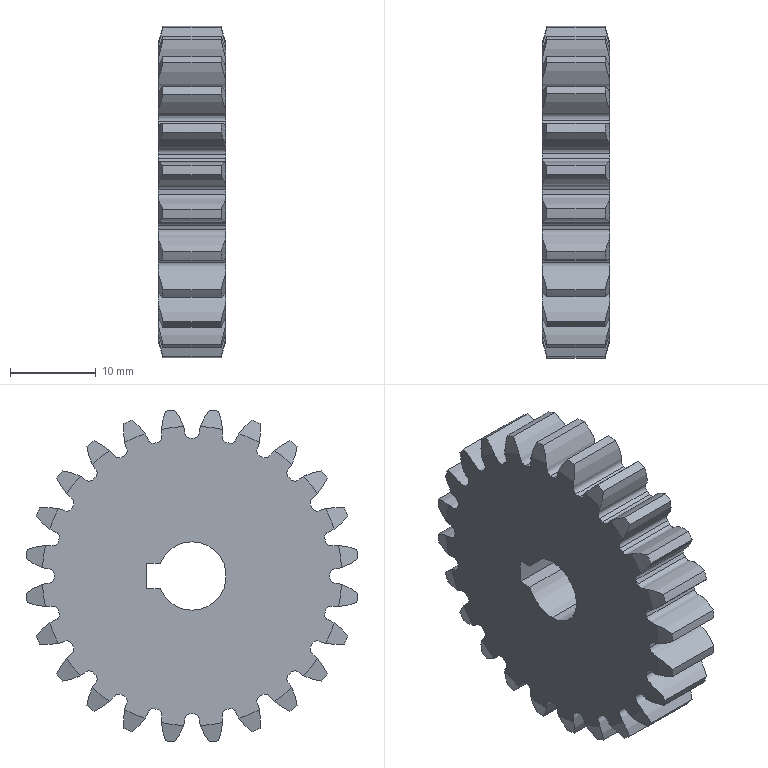Part | SolidWorks | features Chamfer 2, ICE 2, CirPattern 1, Extrusion 1, RefAxis 1 | 1 solid | 152 faces | box 7.851 x 38.792 x 38.792 mm | volume 7390 mm3 | cylinder 51 | spline 48 | cone 48 | plane 5 | commonest cylinder face diameters 32.25 x24 39 x24 8 x3